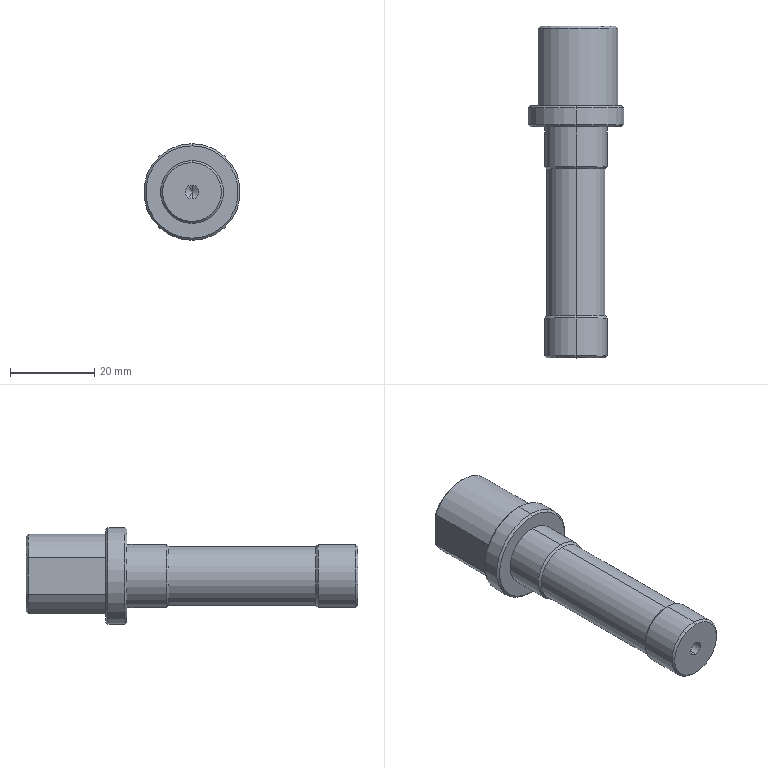Part | STEP file | ND25021-01-JDKM-07-GJ | 1 solid | 34 faces | box 23 x 79 x 23 mm | volume 16613 mm3 | cone 14 | cylinder 12 | plane 8 | commonest cylinder face diameters 15 x4 3.3 x2 14 x2 20 x2 23 x2